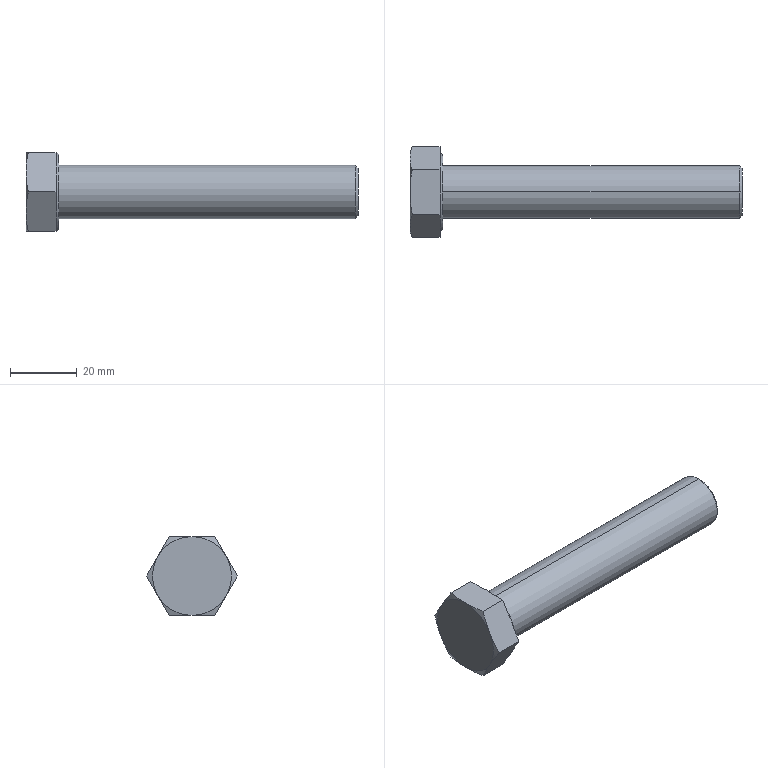Part | STEP file | Hex Head Bolt GB5780-2000 M16(X1.5)X90_GB_FASTENER_BOLT_HHBFPT A M16X1.5X90-N | 1 solid | 27 faces | box 99.82 x 27.332 x 23.67 mm | volume 22788 mm3 | plane 15 | cone 10 | cylinder 2 | commonest cylinder face diameters 16 x2